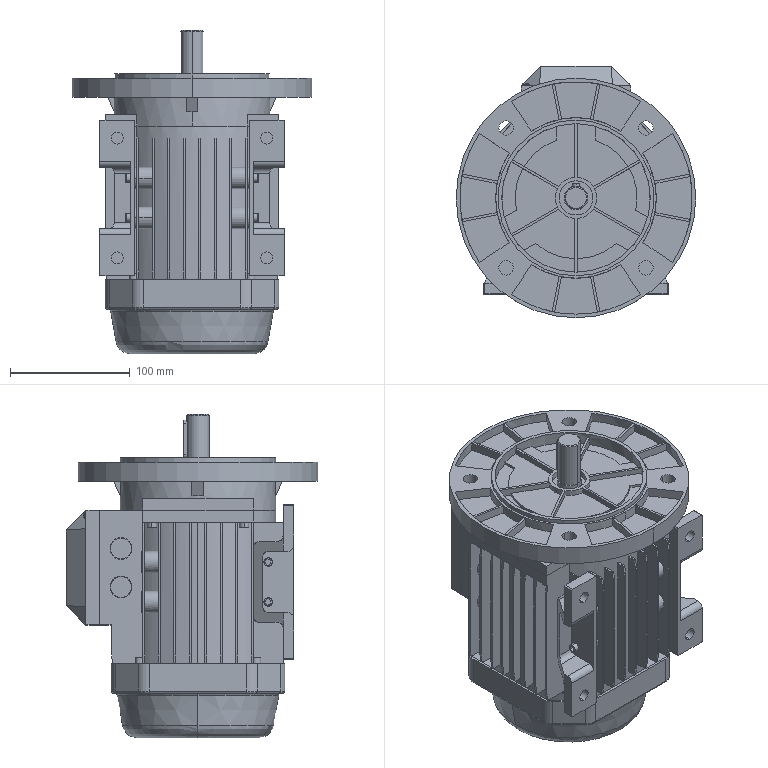Part | SolidWorks | features ICE 42, Fillet 16, MirrorPattern 8, CirPattern 7, Extrusion 5, Revolution 4, Dome 2, LPattern 2, LibraryFeature 2, Chamfer 1, CombineBodies 1, RevCut 1, Shell 1 | 2 solids | 1399 faces | box 200 x 210 x 270 mm | volume 3858118 mm3 | plane 1112 | cylinder 211 | torus 62 | cone 12 | sphere 2 | commonest cylinder face diameters 10 x34 6 x32 18 x26 130 x14 1 x8 2 x8